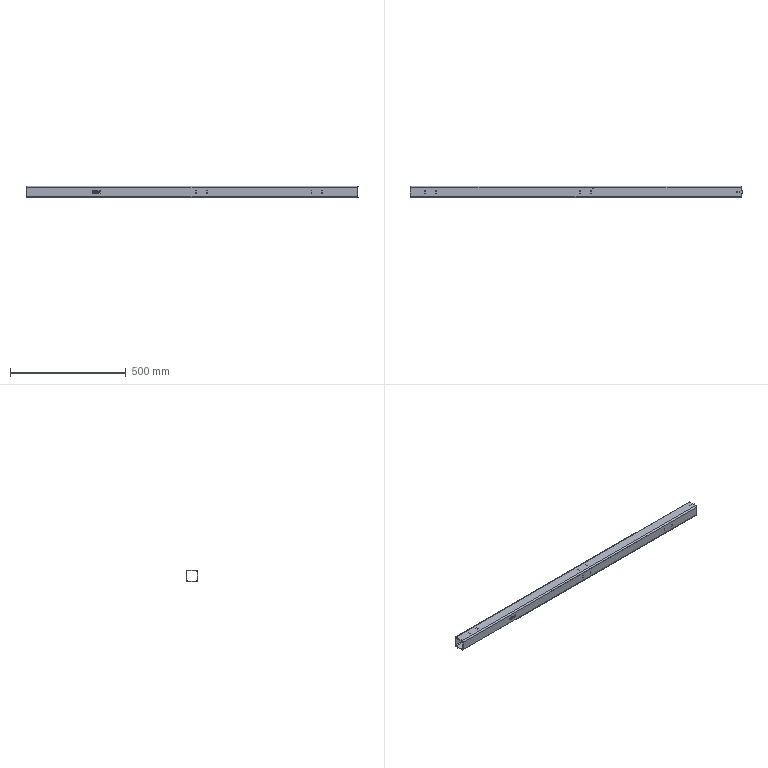Part | SolidWorks | features BaseBody 1 | 1 solid | 129 faces | box 1436 x 50 x 50 mm | volume 769827 mm3 | plane 80 | spline 30 | cylinder 19 | commonest cylinder face diameters 4.2 x10 12 x4 6 x3 5.1 x2